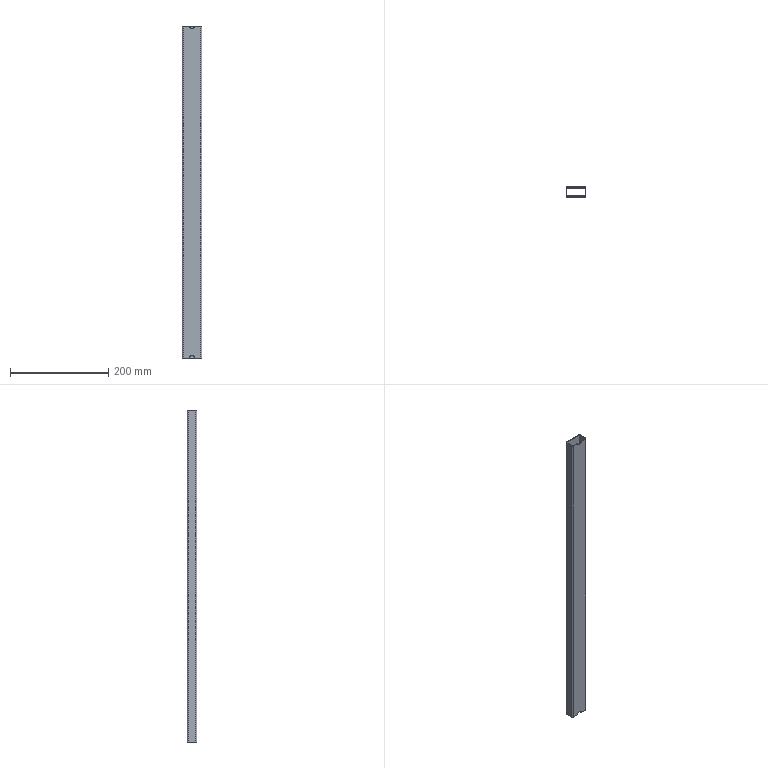Part | STEP file | 6100103 | 1 solid | 20 faces | box 40 x 20 x 675 mm | volume 112265 mm3 | plane 10 | cylinder 10 | commonest cylinder face diameters 2 x4 5 x4 10 x2